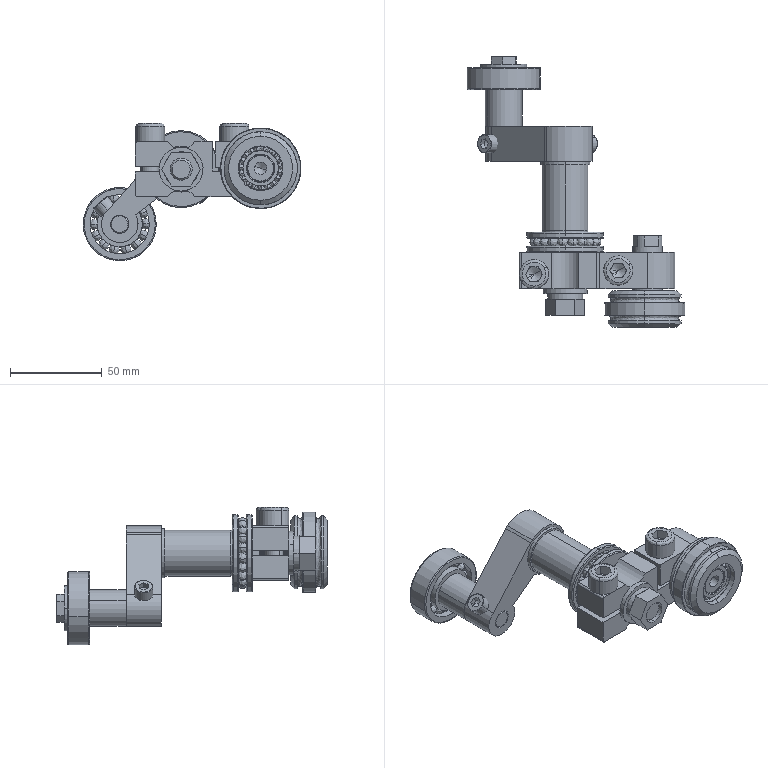Part | SolidWorks | 21 solids | 1267 faces | box 118.949 x 147.9 x 75.017 mm | volume 154608 mm3 | cylinder 477 | spline 403 | plane 351 | cone 36 | commonest cylinder face diameters 0.75 x215 16.285 x95 10 x12 16 x9 19.333 x8 23.667 x8